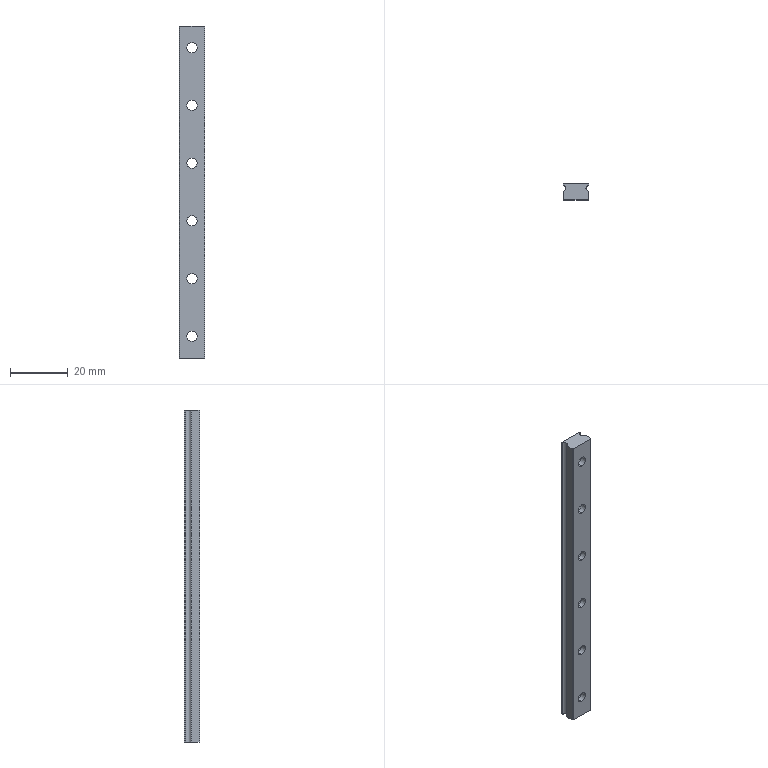Part | SolidWorks | features RefAxis 6, RevCut 6, 3DProfileFeature 2, Extrusion 1 | 1 solid | 43 faces | box 9 x 5.5 x 115 mm | volume 4582 mm3 | cylinder 27 | plane 16 | commonest cylinder face diameters 3.5 x12 6 x12 2.08 x3
STEP:
#1=CARTESIAN_POINT('',(0.,0.,25.75));
#2=VERTEX_POINT('',#1);
#3=CARTESIAN_POINT('',(0.,0.,29.25));
#4=VERTEX_POINT('',#3);
#5=CARTESIAN_POINT('',(0.,0.,27.5));
#6=DIRECTION('',(0.,1.,0.));
#7=DIRECTION('',(0.,0.,1.));
#8=AXIS2_PLACEMENT_3D('',#5,#6,#7);
#9=CIRCLE('',#8,1.75);
#10=EDGE_CURVE('',#2,#4,#9,.T.);
#11=ORIENTED_EDGE('',*,*,#10,.F.);
#12=CARTESIAN_POINT('',(0.,2.,25.75));
#13=VERTEX_POINT('',#12);
#14=CARTESIAN_POINT('',(0.,0.,25.75));
#15=DIRECTION('',(0.,1.,0.));
#16=VECTOR('',#15,1000.);
#17=LINE('',#14,#16);
#18=EDGE_CURVE('',#2,#13,#17,.T.);
#19=ORIENTED_EDGE('',*,*,#18,.T.);
#20=CARTESIAN_POINT('',(0.,2.,29.25));
#21=VERTEX_POINT('',#20);
#22=CARTESIAN_POINT('',(0.,2.,27.5));
#23=DIRECTION('',(0.,1.,0.));
#24=DIRECTION('',(0.,0.,1.));
#25=AXIS2_PLACEMENT_3D('',#22,#23,#24);
#26=CIRCLE('',#25,1.75);
#27=EDGE_CURVE('',#13,#21,#26,.T.);
#28=ORIENTED_EDGE('',*,*,#27,.T.);
#29=CARTESIAN_POINT('',(0.,0.,29.25));
#30=DIRECTION('',(0.,1.,0.));
#31=VECTOR('',#30,1000.);
#32=LINE('',#29,#31);
#33=EDGE_CURVE('',#4,#21,#32,.T.);
#34=ORIENTED_EDGE('',*,*,#33,.F.);
#35=EDGE_LOOP('',(#11,#19,#28,#34));
#36=FACE_OUTER_BOUND('',#35,.T.);
#37=CARTESIAN_POINT('',(0.,0.,27.5));
#38=DIRECTION('',(0.,1.,0.));
#39=DIRECTION('',(0.,0.,1.));
#40=AXIS2_PLACEMENT_3D('',#37,#38,#39);
#41=CYLINDRICAL_SURFACE('',#40,1.75);
#42=ADVANCED_FACE('',(#36),#41,.F.);
#43=CARTESIAN_POINT('',(0.,2.,24.5));
#44=VERTEX_POINT('',#43);
#45=CARTESIAN_POINT('',(0.,2.,30.5));
#46=VERTEX_POINT('',#45);
#47=CARTESIAN_POINT('',(0.,2.,27.5));
#48=DIRECTION('',(0.,1.,0.));
#49=DIRECTION('',(0.,0.,1.));
#50=AXIS2_PLACEMENT_3D('',#47,#48,#49);
#51=CIRCLE('',#50,3.);
#52=EDGE_CURVE('',#44,#46,#51,.T.);
#53=ORIENTED_EDGE('',*,*,#52,.F.);
#54=CARTESIAN_POINT('',(0.,5.5,24.5));
#55=VERTEX_POINT('',#54);
#56=CARTESIAN_POINT('',(0.,0.,24.5));
#57=DIRECTION('',(0.,1.,0.));
#58=VECTOR('',#57,1000.);
#59=LINE('',#56,#58);
#60=EDGE_CURVE('',#44,#55,#59,.T.);
#61=ORIENTED_EDGE('',*,*,#60,.T.);
#62=CARTESIAN_POINT('',(0.,5.5,30.5));
#63=VERTEX_POINT('',#62);
#64=CARTESIAN_POINT('',(0.,5.5,27.5));
#65=DIRECTION('',(0.,1.,0.));
#66=DIRECTION('',(0.,0.,1.));
#67=AXIS2_PLACEMENT_3D('',#64,#65,#66);
#68=CIRCLE('',#67,3.);
#69=EDGE_CURVE('',#55,#63,#68,.T.);
#70=ORIENTED_EDGE('',*,*,#69,.T.);
#71=CARTESIAN_POINT('',(0.,0.,30.5));
#72=DIRECTION('',(0.,1.,0.));
#73=VECTOR('',#72,1000.);
#74=LINE('',#71,#73);
#75=EDGE_CURVE('',#46,#63,#74,.T.);
#76=ORIENTED_EDGE('',*,*,#75,.F.);
#77=EDGE_LOOP('',(#53,#61,#70,#76));
#78=FACE_OUTER_BOUND('',#77,.T.);
#79=CARTESIAN_POINT('',(0.,0.,27.5));
#80=DIRECTION('',(0.,1.,0.));
#81=DIRECTION('',(0.,0.,1.));
#82=AXIS2_PLACEMENT_3D('',#79,#80,#81);
#83=CYLINDRICAL_SURFACE('',#82,3.);
#84=ADVANCED_FACE('',(#78),#83,.F.);
#85=CARTESIAN_POINT('',(0.,0.,45.75));
#86=VERTEX_POINT('',#85);
#87=CARTESIAN_POINT('',(0.,0.,49.25));
#88=VERTEX_POINT('',#87);
#89=CARTESIAN_POINT('',(0.,0.,47.5));
#90=DIRECTION('',(0.,1.,0.));
#91=DIRECTION('',(0.,0.,1.));
#92=AXIS2_PLACEMENT_3D('',#89,#90,#91);
#93=CIRCLE('',#92,1.75);
#94=EDGE_CURVE('',#86,#88,#93,.T.);
#95=ORIENTED_EDGE('',*,*,#94,.F.);
#96=CARTESIAN_POINT('',(0.,2.,45.75));
#97=VERTEX_POINT('',#96);
#98=CARTESIAN_POINT('',(0.,0.,45.75));
#99=DIRECTION('',(0.,1.,0.));
#100=VECTOR('',#99,1000.);
#101=LINE('',#98,#100);
#102=EDGE_CURVE('',#86,#97,#101,.T.);
#103=ORIENTED_EDGE('',*,*,#102,.T.);
#104=CARTESIAN_POINT('',(0.,2.,49.25));
#105=VERTEX_POINT('',#104);
#106=CARTESIAN_POINT('',(0.,2.,47.5));
#107=DIRECTION('',(0.,1.,0.));
#108=DIRECTION('',(0.,0.,1.));
#109=AXIS2_PLACEMENT_3D('',#106,#107,#108);
#110=CIRCLE('',#109,1.75);
#111=EDGE_CURVE('',#97,#105,#110,.T.);
#112=ORIENTED_EDGE('',*,*,#111,.T.);
#113=CARTESIAN_POINT('',(0.,0.,49.25));
#114=DIRECTION('',(0.,1.,0.));
#115=VECTOR('',#114,1000.);
#116=LINE('',#113,#115);
#117=EDGE_CURVE('',#88,#105,#116,.T.);
#118=ORIENTED_EDGE('',*,*,#117,.F.);
#119=EDGE_LOOP('',(#95,#103,#112,#118));
#120=FACE_OUTER_BOUND('',#119,.T.);
#121=CARTESIAN_POINT('',(0.,0.,47.5));
#122=DIRECTION('',(0.,1.,0.));
#123=DIRECTION('',(0.,0.,1.));
#124=AXIS2_PLACEMENT_3D('',#121,#122,#123);
#125=CYLINDRICAL_SURFACE('',#124,1.75);
#126=ADVANCED_FACE('',(#120),#125,.F.);
#127=CARTESIAN_POINT('',(0.,2.,44.5));
#128=VERTEX_POINT('',#127);
#129=CARTESIAN_POINT('',(0.,2.,50.5));
#130=VERTEX_POINT('',#129);
#131=CARTESIAN_POINT('',(0.,2.,47.5));
#132=DIRECTION('',(0.,1.,0.));
#133=DIRECTION('',(0.,0.,1.));
#134=AXIS2_PLACEMENT_3D('',#131,#132,#133);
#135=CIRCLE('',#134,3.);
#136=EDGE_CURVE('',#128,#130,#135,.T.);
#137=ORIENTED_EDGE('',*,*,#136,.F.);
#138=CARTESIAN_POINT('',(0.,5.5,44.5));
#139=VERTEX_POINT('',#138);
#140=CARTESIAN_POINT('',(0.,0.,44.5));
#141=DIRECTION('',(0.,1.,0.));
#142=VECTOR('',#141,1000.);
#143=LINE('',#140,#142);
#144=EDGE_CURVE('',#128,#139,#143,.T.);
#145=ORIENTED_EDGE('',*,*,#144,.T.);
#146=CARTESIAN_POINT('',(0.,5.5,50.5));
#147=VERTEX_POINT('',#146);
#148=CARTESIAN_POINT('',(0.,5.5,47.5));
#149=DIRECTION('',(0.,1.,0.));
#150=DIRECTION('',(0.,0.,1.));
#151=AXIS2_PLACEMENT_3D('',#148,#149,#150);
#152=CIRCLE('',#151,3.);
#153=EDGE_CURVE('',#139,#147,#152,.T.);
#154=ORIENTED_EDGE('',*,*,#153,.T.);
#155=CARTESIAN_POINT('',(0.,0.,50.5));
#156=DIRECTION('',(0.,1.,0.));
#157=VECTOR('',#156,1000.);
#158=LINE('',#155,#157);
#159=EDGE_CURVE('',#130,#147,#158,.T.);
#160=ORIENTED_EDGE('',*,*,#159,.F.);
#161=EDGE_LOOP('',(#137,#145,#154,#160));
#162=FACE_OUTER_BOUND('',#161,.T.);
#163=CARTESIAN_POINT('',(0.,0.,47.5));
#164=DIRECTION('',(0.,1.,0.));
#165=DIRECTION('',(0.,0.,1.));
#166=AXIS2_PLACEMENT_3D('',#163,#164,#165);
#167=CYLINDRICAL_SURFACE('',#166,3.);
#168=ADVANCED_FACE('',(#162),#167,.F.);
#169=CARTESIAN_POINT('',(0.,0.,65.75));
#170=VERTEX_POINT('',#169);
#171=CARTESIAN_POINT('',(0.,0.,69.25));
#172=VERTEX_POINT('',#171);
#173=CARTESIAN_POINT('',(0.,0.,67.5));
#174=DIRECTION('',(0.,1.,0.));
#175=DIRECTION('',(0.,0.,1.));
#176=AXIS2_PLACEMENT_3D('',#173,#174,#175);
#177=CIRCLE('',#176,1.75);
#178=EDGE_CURVE('',#170,#172,#177,.T.);
#179=ORIENTED_EDGE('',*,*,#178,.F.);
#180=CARTESIAN_POINT('',(0.,2.,65.75));
#181=VERTEX_POINT('',#180);
#182=CARTESIAN_POINT('',(0.,0.,65.75));
#183=DIRECTION('',(0.,1.,0.));
#184=VECTOR('',#183,1000.);
#185=LINE('',#182,#184);
#186=EDGE_CURVE('',#170,#181,#185,.T.);
#187=ORIENTED_EDGE('',*,*,#186,.T.);
#188=CARTESIAN_POINT('',(0.,2.,69.25));
#189=VERTEX_POINT('',#188);
#190=CARTESIAN_POINT('',(0.,2.,67.5));
#191=DIRECTION('',(0.,1.,0.));
#192=DIRECTION('',(0.,0.,1.));
#193=AXIS2_PLACEMENT_3D('',#190,#191,#192);
#194=CIRCLE('',#193,1.75);
#195=EDGE_CURVE('',#181,#189,#194,.T.);
#196=ORIENTED_EDGE('',*,*,#195,.T.);
#197=CARTESIAN_POINT('',(0.,0.,69.25));
#198=DIRECTION('',(0.,1.,0.));
#199=VECTOR('',#198,1000.);
#200=LINE('',#197,#199);
#201=EDGE_CURVE('',#172,#189,#200,.T.);
#202=ORIENTED_EDGE('',*,*,#201,.F.);
#203=EDGE_LOOP('',(#179,#187,#196,#202));
#204=FACE_OUTER_BOUND('',#203,.T.);
#205=CARTESIAN_POINT('',(0.,0.,67.5));
#206=DIRECTION('',(0.,1.,0.));
#207=DIRECTION('',(0.,0.,1.));
#208=AXIS2_PLACEMENT_3D('',#205,#206,#207);
#209=CYLINDRICAL_SURFACE('',#208,1.75);
#210=ADVANCED_FACE('',(#204),#209,.F.);
#211=CARTESIAN_POINT('',(0.,2.,64.5));
#212=VERTEX_POINT('',#211);
#213=CARTESIAN_POINT('',(0.,2.,70.5));
#214=VERTEX_POINT('',#213);
#215=CARTESIAN_POINT('',(0.,2.,67.5));
#216=DIRECTION('',(0.,1.,0.));
#217=DIRECTION('',(0.,0.,1.));
#218=AXIS2_PLACEMENT_3D('',#215,#216,#217);
#219=CIRCLE('',#218,3.);
#220=EDGE_CURVE('',#212,#214,#219,.T.);
#221=ORIENTED_EDGE('',*,*,#220,.F.);
#222=CARTESIAN_POINT('',(0.,5.5,64.5));
#223=VERTEX_POINT('',#222);
#224=CARTESIAN_POINT('',(0.,0.,64.5));
#225=DIRECTION('',(0.,1.,0.));
#226=VECTOR('',#225,1000.);
#227=LINE('',#224,#226);
#228=EDGE_CURVE('',#212,#223,#227,.T.);
#229=ORIENTED_EDGE('',*,*,#228,.T.);
#230=CARTESIAN_POINT('',(0.,5.5,70.5));
#231=VERTEX_POINT('',#230);
#232=CARTESIAN_POINT('',(0.,5.5,67.5));
#233=DIRECTION('',(0.,1.,0.));
#234=DIRECTION('',(0.,0.,1.));
#235=AXIS2_PLACEMENT_3D('',#232,#233,#234);
#236=CIRCLE('',#235,3.);
#237=EDGE_CURVE('',#223,#231,#236,.T.);
#238=ORIENTED_EDGE('',*,*,#237,.T.);
#239=CARTESIAN_POINT('',(0.,0.,70.5));
#240=DIRECTION('',(0.,1.,0.));
#241=VECTOR('',#240,1000.);
#242=LINE('',#239,#241);
#243=EDGE_CURVE('',#214,#231,#242,.T.);
#244=ORIENTED_EDGE('',*,*,#243,.F.);
#245=EDGE_LOOP('',(#221,#229,#238,#244));
#246=FACE_OUTER_BOUND('',#245,.T.);
#247=CARTESIAN_POINT('',(0.,0.,67.5));
#248=DIRECTION('',(0.,1.,0.));
#249=DIRECTION('',(0.,0.,1.));
#250=AXIS2_PLACEMENT_3D('',#247,#248,#249);
#251=CYLINDRICAL_SURFACE('',#250,3.);
#252=ADVANCED_FACE('',(#246),#251,.F.);
#253=CARTESIAN_POINT('',(0.,0.,85.75));
#254=VERTEX_POINT('',#253);
#255=CARTESIAN_POINT('',(0.,0.,89.25));
#256=VERTEX_POINT('',#255);
#257=CARTESIAN_POINT('',(0.,0.,87.5));
#258=DIRECTION('',(0.,1.,0.));
#259=DIRECTION('',(0.,0.,1.));
#260=AXIS2_PLACEMENT_3D('',#257,#258,#259);
#261=CIRCLE('',#260,1.75);
#262=EDGE_CURVE('',#254,#256,#261,.T.);
#263=ORIENTED_EDGE('',*,*,#262,.F.);
#264=CARTESIAN_POINT('',(0.,2.,85.75));
#265=VERTEX_POINT('',#264);
#266=CARTESIAN_POINT('',(0.,0.,85.75));
#267=DIRECTION('',(0.,1.,0.));
#268=VECTOR('',#267,1000.);
#269=LINE('',#266,#268);
#270=EDGE_CURVE('',#254,#265,#269,.T.);
#271=ORIENTED_EDGE('',*,*,#270,.T.);
#272=CARTESIAN_POINT('',(0.,2.,89.25));
#273=VERTEX_POINT('',#272);
#274=CARTESIAN_POINT('',(0.,2.,87.5));
#275=DIRECTION('',(0.,1.,0.));
#276=DIRECTION('',(0.,0.,1.));
#277=AXIS2_PLACEMENT_3D('',#274,#275,#276);
#278=CIRCLE('',#277,1.75);
#279=EDGE_CURVE('',#265,#273,#278,.T.);
#280=ORIENTED_EDGE('',*,*,#279,.T.);
#281=CARTESIAN_POINT('',(0.,0.,89.25));
#282=DIRECTION('',(0.,1.,0.));
#283=VECTOR('',#282,1000.);
#284=LINE('',#281,#283);
#285=EDGE_CURVE('',#256,#273,#284,.T.);
#286=ORIENTED_EDGE('',*,*,#285,.F.);
#287=EDGE_LOOP('',(#263,#271,#280,#286));
#288=FACE_OUTER_BOUND('',#287,.T.);
#289=CARTESIAN_POINT('',(0.,0.,87.5));
#290=DIRECTION('',(0.,1.,0.));
#291=DIRECTION('',(0.,0.,1.));
#292=AXIS2_PLACEMENT_3D('',#289,#290,#291);
#293=CYLINDRICAL_SURFACE('',#292,1.75);
#294=ADVANCED_FACE('',(#288),#293,.F.);
#295=CARTESIAN_POINT('',(0.,2.,84.5));
#296=VERTEX_POINT('',#295);
#297=CARTESIAN_POINT('',(0.,2.,90.5));
#298=VERTEX_POINT('',#297);
#299=CARTESIAN_POINT('',(0.,2.,87.5));
#300=DIRECTION('',(0.,1.,0.));
#301=DIRECTION('',(0.,0.,1.));
#302=AXIS2_PLACEMENT_3D('',#299,#300,#301);
#303=CIRCLE('',#302,3.);
#304=EDGE_CURVE('',#296,#298,#303,.T.);
#305=ORIENTED_EDGE('',*,*,#304,.F.);
#306=CARTESIAN_POINT('',(0.,5.5,84.5));
#307=VERTEX_POINT('',#306);
#308=CARTESIAN_POINT('',(0.,0.,84.5));
#309=DIRECTION('',(0.,1.,0.));
#310=VECTOR('',#309,1000.);
#311=LINE('',#308,#310);
#312=EDGE_CURVE('',#296,#307,#311,.T.);
#313=ORIENTED_EDGE('',*,*,#312,.T.);
#314=CARTESIAN_POINT('',(0.,5.5,90.5));
#315=VERTEX_POINT('',#314);
#316=CARTESIAN_POINT('',(0.,5.5,87.5));
#317=DIRECTION('',(0.,1.,0.));
#318=DIRECTION('',(0.,0.,1.));
#319=AXIS2_PLACEMENT_3D('',#316,#317,#318);
#320=CIRCLE('',#319,3.);
#321=EDGE_CURVE('',#307,#315,#320,.T.);
#322=ORIENTED_EDGE('',*,*,#321,.T.);
#323=CARTESIAN_POINT('',(0.,0.,90.5));
#324=DIRECTION('',(0.,1.,0.));
#325=VECTOR('',#324,1000.);
#326=LINE('',#323,#325);
#327=EDGE_CURVE('',#298,#315,#326,.T.);
#328=ORIENTED_EDGE('',*,*,#327,.F.);
#329=EDGE_LOOP('',(#305,#313,#322,#328));
#330=FACE_OUTER_BOUND('',#329,.T.);
#331=CARTESIAN_POINT('',(0.,0.,87.5));
#332=DIRECTION('',(0.,1.,0.));
#333=DIRECTION('',(0.,0.,1.));
#334=AXIS2_PLACEMENT_3D('',#331,#332,#333);
#335=CYLINDRICAL_SURFACE('',#334,3.);
#336=ADVANCED_FACE('',(#330),#335,.F.);
#337=CARTESIAN_POINT('',(0.,0.,105.75));
#338=VERTEX_POINT('',#337);
#339=CARTESIAN_POINT('',(0.,0.,109.25));
#340=VERTEX_POINT('',#339);
#341=CARTESIAN_POINT('',(0.,0.,107.5));
#342=DIRECTION('',(0.,1.,0.));
#343=DIRECTION('',(0.,0.,1.));
#344=AXIS2_PLACEMENT_3D('',#341,#342,#343);
#345=CIRCLE('',#344,1.75);
#346=EDGE_CURVE('',#338,#340,#345,.T.);
#347=ORIENTED_EDGE('',*,*,#346,.F.);
#348=CARTESIAN_POINT('',(0.,2.,105.75));
#349=VERTEX_POINT('',#348);
#350=CARTESIAN_POINT('',(0.,0.,105.75));
#351=DIRECTION('',(0.,1.,0.));
#352=VECTOR('',#351,1000.);
#353=LINE('',#350,#352);
#354=EDGE_CURVE('',#338,#349,#353,.T.);
#355=ORIENTED_EDGE('',*,*,#354,.T.);
#356=CARTESIAN_POINT('',(0.,2.,109.25));
#357=VERTEX_POINT('',#356);
#358=CARTESIAN_POINT('',(0.,2.,107.5));
#359=DIRECTION('',(0.,1.,0.));
#360=DIRECTION('',(0.,0.,1.));
#361=AXIS2_PLACEMENT_3D('',#358,#359,#360);
#362=CIRCLE('',#361,1.75);
#363=EDGE_CURVE('',#349,#357,#362,.T.);
#364=ORIENTED_EDGE('',*,*,#363,.T.);
#365=CARTESIAN_POINT('',(0.,0.,109.25));
#366=DIRECTION('',(0.,1.,0.));
#367=VECTOR('',#366,1000.);
#368=LINE('',#365,#367);
#369=EDGE_CURVE('',#340,#357,#368,.T.);
#370=ORIENTED_EDGE('',*,*,#369,.F.);
#371=EDGE_LOOP('',(#347,#355,#364,#370));
#372=FACE_OUTER_BOUND('',#371,.T.);
#373=CARTESIAN_POINT('',(0.,0.,107.5));
#374=DIRECTION('',(0.,1.,0.));
#375=DIRECTION('',(0.,0.,1.));
#376=AXIS2_PLACEMENT_3D('',#373,#374,#375);
#377=CYLINDRICAL_SURFACE('',#376,1.75);
#378=ADVANCED_FACE('',(#372),#377,.F.);
#379=CARTESIAN_POINT('',(0.,2.,104.5));
#380=VERTEX_POINT('',#379);
#381=CARTESIAN_POINT('',(0.,2.,110.5));
#382=VERTEX_POINT('',#381);
#383=CARTESIAN_POINT('',(0.,2.,107.5));
#384=DIRECTION('',(0.,1.,0.));
#385=DIRECTION('',(0.,0.,1.));
#386=AXIS2_PLACEMENT_3D('',#383,#384,#385);
#387=CIRCLE('',#386,3.);
#388=EDGE_CURVE('',#380,#382,#387,.T.);
#389=ORIENTED_EDGE('',*,*,#388,.F.);
#390=CARTESIAN_POINT('',(0.,5.5,104.5));
#391=VERTEX_POINT('',#390);
#392=CARTESIAN_POINT('',(0.,0.,104.5));
#393=DIRECTION('',(0.,1.,0.));
#394=VECTOR('',#393,1000.);
#395=LINE('',#392,#394);
#396=EDGE_CURVE('',#380,#391,#395,.T.);
#397=ORIENTED_EDGE('',*,*,#396,.T.);
#398=CARTESIAN_POINT('',(0.,5.5,110.5));
#399=VERTEX_POINT('',#398);
#400=CARTESIAN_POINT('',(0.,5.5,107.5));
#401=DIRECTION('',(0.,1.,0.));
#402=DIRECTION('',(0.,0.,1.));
#403=AXIS2_PLACEMENT_3D('',#400,#401,#402);
#404=CIRCLE('',#403,3.);
#405=EDGE_CURVE('',#391,#399,#404,.T.);
#406=ORIENTED_EDGE('',*,*,#405,.T.);
#407=CARTESIAN_POINT('',(0.,0.,110.5));
#408=DIRECTION('',(0.,1.,0.));
#409=VECTOR('',#408,1000.);
#410=LINE('',#407,#409);
#411=EDGE_CURVE('',#382,#399,#410,.T.);
#412=ORIENTED_EDGE('',*,*,#411,.F.);
#413=EDGE_LOOP('',(#389,#397,#406,#412));
#414=FACE_OUTER_BOUND('',#413,.T.);
#415=CARTESIAN_POINT('',(0.,0.,107.5));
#416=DIRECTION('',(0.,1.,0.));
#417=DIRECTION('',(0.,0.,1.));
#418=AXIS2_PLACEMENT_3D('',#415,#416,#417);
#419=CYLINDRICAL_SURFACE('',#418,3.);
#420=ADVANCED_FACE('',(#414),#419,.F.);
#421=CARTESIAN_POINT('',(0.,0.,5.75));
#422=VERTEX_POINT('',#421);
#423=CARTESIAN_POINT('',(0.,0.,9.25));
#424=VERTEX_POINT('',#423);
#425=CARTESIAN_POINT('',(0.,0.,7.5));
#426=DIRECTION('',(0.,1.,0.));
#427=DIRECTION('',(0.,0.,1.));
#428=AXIS2_PLACEMENT_3D('',#425,#426,#427);
#429=CIRCLE('',#428,1.75);
#430=EDGE_CURVE('',#422,#424,#429,.T.);
#431=ORIENTED_EDGE('',*,*,#430,.F.);
#432=CARTESIAN_POINT('',(0.,2.,5.75));
#433=VERTEX_POINT('',#432);
#434=CARTESIAN_POINT('',(0.,0.,5.75));
#435=DIRECTION('',(0.,1.,0.));
#436=VECTOR('',#435,1000.);
#437=LINE('',#434,#436);
#438=EDGE_CURVE('',#422,#433,#437,.T.);
#439=ORIENTED_EDGE('',*,*,#438,.T.);
#440=CARTESIAN_POINT('',(0.,2.,9.25));
#441=VERTEX_POINT('',#440);
#442=CARTESIAN_POINT('',(0.,2.,7.5));
#443=DIRECTION('',(0.,1.,0.));
#444=DIRECTION('',(0.,0.,1.));
#445=AXIS2_PLACEMENT_3D('',#442,#443,#444);
#446=CIRCLE('',#445,1.75);
#447=EDGE_CURVE('',#433,#441,#446,.T.);
#448=ORIENTED_EDGE('',*,*,#447,.T.);
#449=CARTESIAN_POINT('',(0.,0.,9.25));
#450=DIRECTION('',(0.,1.,0.));
#451=VECTOR('',#450,1000.);
#452=LINE('',#449,#451);
#453=EDGE_CURVE('',#424,#441,#452,.T.);
#454=ORIENTED_EDGE('',*,*,#453,.F.);
#455=EDGE_LOOP('',(#431,#439,#448,#454));
#456=FACE_OUTER_BOUND('',#455,.T.);
#457=CARTESIAN_POINT('',(0.,0.,7.5));
#458=DIRECTION('',(0.,1.,0.));
#459=DIRECTION('',(0.,0.,1.));
#460=AXIS2_PLACEMENT_3D('',#457,#458,#459);
#461=CYLINDRICAL_SURFACE('',#460,1.75);
#462=ADVANCED_FACE('',(#456),#461,.F.);
#463=CARTESIAN_POINT('',(0.,2.,4.5));
#464=VERTEX_POINT('',#463);
#465=CARTESIAN_POINT('',(0.,2.,10.5));
#466=VERTEX_POINT('',#465);
#467=CARTESIAN_POINT('',(0.,2.,7.5));
#468=DIRECTION('',(0.,1.,0.));
#469=DIRECTION('',(0.,0.,1.));
#470=AXIS2_PLACEMENT_3D('',#467,#468,#469);
#471=CIRCLE('',#470,3.);
#472=EDGE_CURVE('',#464,#466,#471,.T.);
#473=ORIENTED_EDGE('',*,*,#472,.F.);
#474=CARTESIAN_POINT('',(0.,5.5,4.5));
#475=VERTEX_POINT('',#474);
#476=CARTESIAN_POINT('',(0.,0.,4.5));
#477=DIRECTION('',(0.,1.,0.));
#478=VECTOR('',#477,1000.);
#479=LINE('',#476,#478);
#480=EDGE_CURVE('',#464,#475,#479,.T.);
#481=ORIENTED_EDGE('',*,*,#480,.T.);
#482=CARTESIAN_POINT('',(0.,5.5,10.5));
#483=VERTEX_POINT('',#482);
#484=CARTESIAN_POINT('',(0.,5.5,7.5));
#485=DIRECTION('',(0.,1.,0.));
#486=DIRECTION('',(0.,0.,1.));
#487=AXIS2_PLACEMENT_3D('',#484,#485,#486);
#488=CIRCLE('',#487,3.);
#489=EDGE_CURVE('',#475,#483,#488,.T.);
#490=ORIENTED_EDGE('',*,*,#489,.T.);
#491=CARTESIAN_POINT('',(0.,0.,10.5));
#492=DIRECTION('',(0.,1.,0.));
#493=VECTOR('',#492,1000.);
#494=LINE('',#491,#493);
#495=EDGE_CURVE('',#466,#483,#494,.T.);
#496=ORIENTED_EDGE('',*,*,#495,.F.);
#497=EDGE_LOOP('',(#473,#481,#490,#496));
#498=FACE_OUTER_BOUND('',#497,.T.);
#499=CARTESIAN_POINT('',(0.,0.,7.5));
#500=DIRECTION('',(0.,1.,0.));
#501=DIRECTION('',(0.,0.,1.));
#502=AXIS2_PLACEMENT_3D('',#499,#500,#501);
#503=CYLINDRICAL_SURFACE('',#502,3.);
#504=ADVANCED_FACE('',(#498),#503,.F.);
#505=CARTESIAN_POINT('',(3.46,4.,115.));
#506=VERTEX_POINT('',#505);
#507=CARTESIAN_POINT('',(4.5,5.04,115.));
#508=VERTEX_POINT('',#507);
#509=CARTESIAN_POINT('',(4.5,4.,115.));
#510=DIRECTION('',(0.,0.,-1.));
#511=DIRECTION('',(-1.,0.,0.));
#512=AXIS2_PLACEMENT_3D('',#509,#510,#511);
#513=CIRCLE('',#512,1.04);
#514=EDGE_CURVE('',#506,#508,#513,.T.);
#515=ORIENTED_EDGE('',*,*,#514,.F.);
#516=CARTESIAN_POINT('',(3.46,4.,0.));
#517=VERTEX_POINT('',#516);
#518=CARTESIAN_POINT('',(3.46,4.,115.));
#519=DIRECTION('',(0.,0.,-1.));
#520=VECTOR('',#519,1000.);
#521=LINE('',#518,#520);
#522=EDGE_CURVE('',#506,#517,#521,.T.);
#523=ORIENTED_EDGE('',*,*,#522,.T.);
#524=CARTESIAN_POINT('',(4.5,5.04,0.));
#525=VERTEX_POINT('',#524);
#526=CARTESIAN_POINT('',(4.5,4.,0.));
#527=DIRECTION('',(0.,0.,-1.));
#528=DIRECTION('',(-1.,0.,0.));
#529=AXIS2_PLACEMENT_3D('',#526,#527,#528);
#530=CIRCLE('',#529,1.04);
#531=EDGE_CURVE('',#517,#525,#530,.T.);
#532=ORIENTED_EDGE('',*,*,#531,.T.);
#533=CARTESIAN_POINT('',(4.5,5.04,115.));
#534=DIRECTION('',(0.,0.,-1.));
#535=VECTOR('',#534,1000.);
#536=LINE('',#533,#535);
#537=EDGE_CURVE('',#508,#525,#536,.T.);
#538=ORIENTED_EDGE('',*,*,#537,.F.);
#539=EDGE_LOOP('',(#515,#523,#532,#538));
#540=FACE_OUTER_BOUND('',#539,.T.);
#541=CARTESIAN_POINT('',(4.5,4.,115.));
#542=DIRECTION('',(0.,0.,-1.));
#543=DIRECTION('',(-1.,0.,0.));
#544=AXIS2_PLACEMENT_3D('',#541,#542,#543);
#545=CYLINDRICAL_SURFACE('',#544,1.04);
#546=ADVANCED_FACE('',(#540),#545,.F.);
#547=CARTESIAN_POINT('',(0.,5.5,47.5));
#548=DIRECTION('',(0.,1.,0.));
#549=DIRECTION('',(0.,0.,1.));
#550=AXIS2_PLACEMENT_3D('',#547,#548,#549);
#551=CIRCLE('',#550,3.);
#552=EDGE_CURVE('',#147,#139,#551,.T.);
#553=ORIENTED_EDGE('',*,*,#552,.F.);
#554=ORIENTED_EDGE('',*,*,#153,.F.);
#555=EDGE_LOOP('',(#553,#554));
#556=FACE_BOUND('',#555,.T.);
#557=CARTESIAN_POINT('',(0.,5.5,87.5));
#558=DIRECTION('',(0.,1.,0.));
#559=DIRECTION('',(0.,0.,1.));
#560=AXIS2_PLACEMENT_3D('',#557,#558,#559);
#561=CIRCLE('',#560,3.);
#562=EDGE_CURVE('',#315,#307,#561,.T.);
#563=ORIENTED_EDGE('',*,*,#562,.F.);
#564=ORIENTED_EDGE('',*,*,#321,.F.);
#565=EDGE_LOOP('',(#563,#564));
#566=FACE_BOUND('',#565,.T.);
#567=CARTESIAN_POINT('',(0.,5.5,7.5));
#568=DIRECTION('',(0.,1.,0.));
#569=DIRECTION('',(0.,0.,1.));
#570=AXIS2_PLACEMENT_3D('',#567,#568,#569);
#571=CIRCLE('',#570,3.);
#572=EDGE_CURVE('',#483,#475,#571,.T.);
#573=ORIENTED_EDGE('',*,*,#572,.F.);
#574=ORIENTED_EDGE('',*,*,#489,.F.);
#575=EDGE_LOOP('',(#573,#574));
#576=FACE_BOUND('',#575,.T.);
#577=CARTESIAN_POINT('',(4.5,5.5,0.));
#578=VERTEX_POINT('',#577);
#579=CARTESIAN_POINT('',(-4.5,5.5,0.));
#580=VERTEX_POINT('',#579);
#581=CARTESIAN_POINT('',(4.5,5.5,0.));
#582=DIRECTION('',(-1.,0.,0.));
#583=VECTOR('',#582,1000.);
#584=LINE('',#581,#583);
#585=EDGE_CURVE('',#578,#580,#584,.T.);
#586=ORIENTED_EDGE('',*,*,#585,.T.);
#587=CARTESIAN_POINT('',(-4.5,5.5,115.));
#588=VERTEX_POINT('',#587);
#589=CARTESIAN_POINT('',(-4.5,5.5,115.));
#590=DIRECTION('',(0.,0.,-1.));
#591=VECTOR('',#590,1000.);
#592=LINE('',#589,#591);
#593=EDGE_CURVE('',#588,#580,#592,.T.);
#594=ORIENTED_EDGE('',*,*,#593,.F.);
#595=CARTESIAN_POINT('',(4.5,5.5,115.));
#596=VERTEX_POINT('',#595);
#597=CARTESIAN_POINT('',(4.5,5.5,115.));
#598=DIRECTION('',(-1.,0.,0.));
#599=VECTOR('',#598,1000.);
#600=LINE('',#597,#599);
#601=EDGE_CURVE('',#596,#588,#600,.T.);
#602=ORIENTED_EDGE('',*,*,#601,.F.);
#603=CARTESIAN_POINT('',(4.5,5.5,115.));
#604=DIRECTION('',(0.,0.,-1.));
#605=VECTOR('',#604,1000.);
#606=LINE('',#603,#605);
#607=EDGE_CURVE('',#596,#578,#606,.T.);
#608=ORIENTED_EDGE('',*,*,#607,.T.);
#609=EDGE_LOOP('',(#586,#594,#602,#608));
#610=FACE_OUTER_BOUND('',#609,.T.);
#611=CARTESIAN_POINT('',(0.,5.5,107.5));
#612=DIRECTION('',(0.,1.,0.));
#613=DIRECTION('',(0.,0.,1.));
#614=AXIS2_PLACEMENT_3D('',#611,#612,#613);
#615=CIRCLE('',#614,3.);
#616=EDGE_CURVE('',#399,#391,#615,.T.);
#617=ORIENTED_EDGE('',*,*,#616,.F.);
#618=ORIENTED_EDGE('',*,*,#405,.F.);
#619=EDGE_LOOP('',(#617,#618));
#620=FACE_BOUND('',#619,.T.);
#621=CARTESIAN_POINT('',(0.,5.5,67.5));
#622=DIRECTION('',(0.,1.,0.));
#623=DIRECTION('',(0.,0.,1.));
#624=AXIS2_PLACEMENT_3D('',#621,#622,#623);
#625=CIRCLE('',#624,3.);
#626=EDGE_CURVE('',#231,#223,#625,.T.);
#627=ORIENTED_EDGE('',*,*,#626,.F.);
#628=ORIENTED_EDGE('',*,*,#237,.F.);
#629=EDGE_LOOP('',(#627,#628));
#630=FACE_BOUND('',#629,.T.);
#631=CARTESIAN_POINT('',(0.,5.5,27.5));
#632=DIRECTION('',(0.,1.,0.));
#633=DIRECTION('',(0.,0.,1.));
#634=AXIS2_PLACEMENT_3D('',#631,#632,#633);
#635=CIRCLE('',#634,3.);
#636=EDGE_CURVE('',#63,#55,#635,.T.);
#637=ORIENTED_EDGE('',*,*,#636,.F.);
#638=ORIENTED_EDGE('',*,*,#69,.F.);
#639=EDGE_LOOP('',(#637,#638));
#640=FACE_BOUND('',#639,.T.);
#641=CARTESIAN_POINT('',(4.5,5.5,115.));
#642=DIRECTION('',(0.,-1.,0.));
#643=DIRECTION('',(0.,0.,-1.));
#644=AXIS2_PLACEMENT_3D('',#641,#642,#643);
#645=PLANE('',#644);
#646=ADVANCED_FACE('',(#556,#566,#576,#610,#620,#630,#640),#645,.F.);
#647=CARTESIAN_POINT('',(0.,0.,47.5));
#648=DIRECTION('',(0.,1.,0.));
#649=DIRECTION('',(0.,0.,1.));
#650=AXIS2_PLACEMENT_3D('',#647,#648,#649);
#651=CIRCLE('',#650,1.75);
#652=EDGE_CURVE('',#88,#86,#651,.T.);
#653=ORIENTED_EDGE('',*,*,#652,.T.);
#654=ORIENTED_EDGE('',*,*,#94,.T.);
#655=EDGE_LOOP('',(#653,#654));
#656=FACE_BOUND('',#655,.T.);
#657=CARTESIAN_POINT('',(0.,0.,87.5));
#658=DIRECTION('',(0.,1.,0.));
#659=DIRECTION('',(0.,0.,1.));
#660=AXIS2_PLACEMENT_3D('',#657,#658,#659);
#661=CIRCLE('',#660,1.75);
#662=EDGE_CURVE('',#256,#254,#661,.T.);
#663=ORIENTED_EDGE('',*,*,#662,.T.);
#664=ORIENTED_EDGE('',*,*,#262,.T.);
#665=EDGE_LOOP('',(#663,#664));
#666=FACE_BOUND('',#665,.T.);
#667=CARTESIAN_POINT('',(0.,0.,7.5));
#668=DIRECTION('',(0.,1.,0.));
#669=DIRECTION('',(0.,0.,1.));
#670=AXIS2_PLACEMENT_3D('',#667,#668,#669);
#671=CIRCLE('',#670,1.75);
#672=EDGE_CURVE('',#424,#422,#671,.T.);
#673=ORIENTED_EDGE('',*,*,#672,.T.);
#674=ORIENTED_EDGE('',*,*,#430,.T.);
#675=EDGE_LOOP('',(#673,#674));
#676=FACE_BOUND('',#675,.T.);
#677=CARTESIAN_POINT('',(-4.203,0.,0.));
#678=VERTEX_POINT('',#677);
#679=CARTESIAN_POINT('',(4.203,0.,0.));
#680=VERTEX_POINT('',#679);
#681=CARTESIAN_POINT('',(-4.203,0.,0.));
#682=DIRECTION('',(1.,0.,0.));
#683=VECTOR('',#682,1000.);
#684=LINE('',#681,#683);
#685=EDGE_CURVE('',#678,#680,#684,.T.);
#686=ORIENTED_EDGE('',*,*,#685,.T.);
#687=CARTESIAN_POINT('',(4.203,0.,115.));
#688=VERTEX_POINT('',#687);
#689=CARTESIAN_POINT('',(4.203,0.,115.));
#690=DIRECTION('',(0.,0.,-1.));
#691=VECTOR('',#690,1000.);
#692=LINE('',#689,#691);
#693=EDGE_CURVE('',#688,#680,#692,.T.);
#694=ORIENTED_EDGE('',*,*,#693,.F.);
#695=CARTESIAN_POINT('',(-4.203,0.,115.));
#696=VERTEX_POINT('',#695);
#697=CARTESIAN_POINT('',(-4.203,0.,115.));
#698=DIRECTION('',(1.,0.,0.));
#699=VECTOR('',#698,1000.);
#700=LINE('',#697,#699);
#701=EDGE_CURVE('',#696,#688,#700,.T.);
#702=ORIENTED_EDGE('',*,*,#701,.F.);
#703=CARTESIAN_POINT('',(-4.203,0.,115.));
#704=DIRECTION('',(0.,0.,-1.));
#705=VECTOR('',#704,1000.);
#706=LINE('',#703,#705);
#707=EDGE_CURVE('',#696,#678,#706,.T.);
#708=ORIENTED_EDGE('',*,*,#707,.T.);
#709=EDGE_LOOP('',(#686,#694,#702,#708));
#710=FACE_OUTER_BOUND('',#709,.T.);
#711=CARTESIAN_POINT('',(0.,0.,107.5));
#712=DIRECTION('',(0.,1.,0.));
#713=DIRECTION('',(0.,0.,1.));
#714=AXIS2_PLACEMENT_3D('',#711,#712,#713);
#715=CIRCLE('',#714,1.75);
#716=EDGE_CURVE('',#340,#338,#715,.T.);
#717=ORIENTED_EDGE('',*,*,#716,.T.);
#718=ORIENTED_EDGE('',*,*,#346,.T.);
#719=EDGE_LOOP('',(#717,#718));
#720=FACE_BOUND('',#719,.T.);
#721=CARTESIAN_POINT('',(0.,0.,67.5));
#722=DIRECTION('',(0.,1.,0.));
#723=DIRECTION('',(0.,0.,1.));
#724=AXIS2_PLACEMENT_3D('',#721,#722,#723);
#725=CIRCLE('',#724,1.75);
#726=EDGE_CURVE('',#172,#170,#725,.T.);
#727=ORIENTED_EDGE('',*,*,#726,.T.);
#728=ORIENTED_EDGE('',*,*,#178,.T.);
#729=EDGE_LOOP('',(#727,#728));
#730=FACE_BOUND('',#729,.T.);
#731=CARTESIAN_POINT('',(0.,0.,27.5));
#732=DIRECTION('',(0.,1.,0.));
#733=DIRECTION('',(0.,0.,1.));
#734=AXIS2_PLACEMENT_3D('',#731,#732,#733);
#735=CIRCLE('',#734,1.75);
#736=EDGE_CURVE('',#4,#2,#735,.T.);
#737=ORIENTED_EDGE('',*,*,#736,.T.);
#738=ORIENTED_EDGE('',*,*,#10,.T.);
#739=EDGE_LOOP('',(#737,#738));
#740=FACE_BOUND('',#739,.T.);
#741=CARTESIAN_POINT('',(-4.203,0.,115.));
#742=DIRECTION('',(0.,1.,0.));
#743=DIRECTION('',(0.,0.,1.));
#744=AXIS2_PLACEMENT_3D('',#741,#742,#743);
#745=PLANE('',#744);
#746=ADVANCED_FACE('',(#656,#666,#676,#710,#720,#730,#740),#745,.F.);
#747=CARTESIAN_POINT('',(-4.5,5.04,0.));
#748=VERTEX_POINT('',#747);
#749=CARTESIAN_POINT('',(-4.5,5.5,0.));
#750=DIRECTION('',(0.,-1.,0.));
#751=VECTOR('',#750,1000.);
#752=LINE('',#749,#751);
#753=EDGE_CURVE('',#580,#748,#752,.T.);
#754=ORIENTED_EDGE('',*,*,#753,.T.);
#755=CARTESIAN_POINT('',(-4.5,5.04,115.));
#756=VERTEX_POINT('',#755);
#757=CARTESIAN_POINT('',(-4.5,5.04,115.));
#758=DIRECTION('',(0.,0.,-1.));
#759=VECTOR('',#758,1000.);
#760=LINE('',#757,#759);
#761=EDGE_CURVE('',#756,#748,#760,.T.);
#762=ORIENTED_EDGE('',*,*,#761,.F.);
#763=CARTESIAN_POINT('',(-4.5,5.5,115.));
#764=DIRECTION('',(0.,-1.,0.));
#765=VECTOR('',#764,1000.);
#766=LINE('',#763,#765);
#767=EDGE_CURVE('',#588,#756,#766,.T.);
#768=ORIENTED_EDGE('',*,*,#767,.F.);
#769=ORIENTED_EDGE('',*,*,#593,.T.);
#770=EDGE_LOOP('',(#754,#762,#768,#769));
#771=FACE_OUTER_BOUND('',#770,.T.);
#772=CARTESIAN_POINT('',(-4.5,5.5,115.));
#773=DIRECTION('',(1.,0.,0.));
#774=DIRECTION('',(0.,0.,-1.));
#775=AXIS2_PLACEMENT_3D('',#772,#773,#774);
#776=PLANE('',#775);
#777=ADVANCED_FACE('',(#771),#776,.F.);
#778=CARTESIAN_POINT('',(-4.5,2.96,0.));
#779=VERTEX_POINT('',#778);
#780=CARTESIAN_POINT('',(-4.5,4.,0.));
#781=DIRECTION('',(0.,0.,-1.));
#782=DIRECTION('',(-1.,0.,0.));
#783=AXIS2_PLACEMENT_3D('',#780,#781,#782);
#784=CIRCLE('',#783,1.04);
#785=EDGE_CURVE('',#748,#779,#784,.T.);
#786=ORIENTED_EDGE('',*,*,#785,.T.);
#787=CARTESIAN_POINT('',(-4.5,2.96,115.));
#788=VERTEX_POINT('',#787);
#789=CARTESIAN_POINT('',(-4.5,2.96,115.));
#790=DIRECTION('',(0.,0.,-1.));
#791=VECTOR('',#790,1000.);
#792=LINE('',#789,#791);
#793=EDGE_CURVE('',#788,#779,#792,.T.);
#794=ORIENTED_EDGE('',*,*,#793,.F.);
#795=CARTESIAN_POINT('',(-4.5,4.,115.));
#796=DIRECTION('',(0.,0.,-1.));
#797=DIRECTION('',(-1.,0.,0.));
#798=AXIS2_PLACEMENT_3D('',#795,#796,#797);
#799=CIRCLE('',#798,1.04);
#800=EDGE_CURVE('',#756,#788,#799,.T.);
#801=ORIENTED_EDGE('',*,*,#800,.F.);
#802=ORIENTED_EDGE('',*,*,#761,.T.);
#803=EDGE_LOOP('',(#786,#794,#801,#802));
#804=FACE_OUTER_BOUND('',#803,.T.);
#805=CARTESIAN_POINT('',(-4.5,4.,115.));
#806=DIRECTION('',(0.,0.,-1.));
#807=DIRECTION('',(-1.,0.,0.));
#808=AXIS2_PLACEMENT_3D('',#805,#806,#807);
#809=CYLINDRICAL_SURFACE('',#808,1.04);
#810=ADVANCED_FACE('',(#804),#809,.F.);
#811=CARTESIAN_POINT('',(-4.5,0.297,0.));
#812=VERTEX_POINT('',#811);
#813=CARTESIAN_POINT('',(-4.5,2.96,0.));
#814=DIRECTION('',(0.,-1.,0.));
#815=VECTOR('',#814,1000.);
#816=LINE('',#813,#815);
#817=EDGE_CURVE('',#779,#812,#816,.T.);
#818=ORIENTED_EDGE('',*,*,#817,.T.);
#819=CARTESIAN_POINT('',(-4.5,0.297,115.));
#820=VERTEX_POINT('',#819);
#821=CARTESIAN_POINT('',(-4.5,0.297,115.));
#822=DIRECTION('',(0.,0.,-1.));
#823=VECTOR('',#822,1000.);
#824=LINE('',#821,#823);
#825=EDGE_CURVE('',#820,#812,#824,.T.);
#826=ORIENTED_EDGE('',*,*,#825,.F.);
#827=CARTESIAN_POINT('',(-4.5,2.96,115.));
#828=DIRECTION('',(0.,-1.,0.));
#829=VECTOR('',#828,1000.);
#830=LINE('',#827,#829);
#831=EDGE_CURVE('',#788,#820,#830,.T.);
#832=ORIENTED_EDGE('',*,*,#831,.F.);
#833=ORIENTED_EDGE('',*,*,#793,.T.);
#834=EDGE_LOOP('',(#818,#826,#832,#833));
#835=FACE_OUTER_BOUND('',#834,.T.);
#836=CARTESIAN_POINT('',(-4.5,2.96,115.));
#837=DIRECTION('',(1.,0.,0.));
#838=DIRECTION('',(0.,0.,-1.));
#839=AXIS2_PLACEMENT_3D('',#836,#837,#838);
#840=PLANE('',#839);
#841=ADVANCED_FACE('',(#835),#840,.F.);
#842=CARTESIAN_POINT('',(-4.5,0.297,0.));
#843=DIRECTION('',(0.7071,-0.7071,0.));
#844=VECTOR('',#843,1000.);
#845=LINE('',#842,#844);
#846=EDGE_CURVE('',#812,#678,#845,.T.);
#847=ORIENTED_EDGE('',*,*,#846,.T.);
#848=ORIENTED_EDGE('',*,*,#707,.F.);
#849=CARTESIAN_POINT('',(-4.5,0.297,115.));
#850=DIRECTION('',(0.7071,-0.7071,0.));
#851=VECTOR('',#850,1000.);
#852=LINE('',#849,#851);
#853=EDGE_CURVE('',#820,#696,#852,.T.);
#854=ORIENTED_EDGE('',*,*,#853,.F.);
#855=ORIENTED_EDGE('',*,*,#825,.T.);
#856=EDGE_LOOP('',(#847,#848,#854,#855));
#857=FACE_OUTER_BOUND('',#856,.T.);
#858=CARTESIAN_POINT('',(-4.5,0.297,115.));
#859=DIRECTION('',(0.7071,0.7071,0.));
#860=DIRECTION('',(-0.7071,0.7071,0.));
#861=AXIS2_PLACEMENT_3D('',#858,#859,#860);
#862=PLANE('',#861);
#863=ADVANCED_FACE('',(#857),#862,.F.);
#864=CARTESIAN_POINT('',(4.5,0.297,0.));
#865=VERTEX_POINT('',#864);
#866=CARTESIAN_POINT('',(4.203,0.,0.));
#867=DIRECTION('',(0.7071,0.7071,0.));
#868=VECTOR('',#867,1000.);
#869=LINE('',#866,#868);
#870=EDGE_CURVE('',#680,#865,#869,.T.);
#871=ORIENTED_EDGE('',*,*,#870,.T.);
#872=CARTESIAN_POINT('',(4.5,0.297,115.));
#873=VERTEX_POINT('',#872);
#874=CARTESIAN_POINT('',(4.5,0.297,115.));
#875=DIRECTION('',(0.,0.,-1.));
#876=VECTOR('',#875,1000.);
#877=LINE('',#874,#876);
#878=EDGE_CURVE('',#873,#865,#877,.T.);
#879=ORIENTED_EDGE('',*,*,#878,.F.);
#880=CARTESIAN_POINT('',(4.203,0.,115.));
#881=DIRECTION('',(0.7071,0.7071,0.));
#882=VECTOR('',#881,1000.);
#883=LINE('',#880,#882);
#884=EDGE_CURVE('',#688,#873,#883,.T.);
#885=ORIENTED_EDGE('',*,*,#884,.F.);
#886=ORIENTED_EDGE('',*,*,#693,.T.);
#887=EDGE_LOOP('',(#871,#879,#885,#886));
#888=FACE_OUTER_BOUND('',#887,.T.);
#889=CARTESIAN_POINT('',(4.203,0.,115.));
#890=DIRECTION('',(-0.7071,0.7071,0.));
#891=DIRECTION('',(-0.7071,-0.7071,0.));
#892=AXIS2_PLACEMENT_3D('',#889,#890,#891);
#893=PLANE('',#892);
#894=ADVANCED_FACE('',(#888),#893,.F.);
#895=CARTESIAN_POINT('',(4.5,2.96,0.));
#896=VERTEX_POINT('',#895);
#897=CARTESIAN_POINT('',(4.5,0.297,0.));
#898=DIRECTION('',(0.,1.,0.));
#899=VECTOR('',#898,1000.);
#900=LINE('',#897,#899);
#901=EDGE_CURVE('',#865,#896,#900,.T.);
#902=ORIENTED_EDGE('',*,*,#901,.T.);
#903=CARTESIAN_POINT('',(4.5,2.96,115.));
#904=VERTEX_POINT('',#903);
#905=CARTESIAN_POINT('',(4.5,2.96,115.));
#906=DIRECTION('',(0.,0.,-1.));
#907=VECTOR('',#906,1000.);
#908=LINE('',#905,#907);
#909=EDGE_CURVE('',#904,#896,#908,.T.);
#910=ORIENTED_EDGE('',*,*,#909,.F.);
#911=CARTESIAN_POINT('',(4.5,0.297,115.));
#912=DIRECTION('',(0.,1.,0.));
#913=VECTOR('',#912,1000.);
#914=LINE('',#911,#913);
#915=EDGE_CURVE('',#873,#904,#914,.T.);
#916=ORIENTED_EDGE('',*,*,#915,.F.);
#917=ORIENTED_EDGE('',*,*,#878,.T.);
#918=EDGE_LOOP('',(#902,#910,#916,#917));
#919=FACE_OUTER_BOUND('',#918,.T.);
#920=CARTESIAN_POINT('',(4.5,0.297,115.));
#921=DIRECTION('',(-1.,0.,0.));
#922=DIRECTION('',(0.,0.,1.));
#923=AXIS2_PLACEMENT_3D('',#920,#921,#922);
#924=PLANE('',#923);
#925=ADVANCED_FACE('',(#919),#924,.F.);
#926=ORIENTED_EDGE('',*,*,#522,.F.);
#927=CARTESIAN_POINT('',(4.5,4.,115.));
#928=DIRECTION('',(0.,0.,-1.));
#929=DIRECTION('',(-1.,0.,0.));
#930=AXIS2_PLACEMENT_3D('',#927,#928,#929);
#931=CIRCLE('',#930,1.04);
#932=EDGE_CURVE('',#904,#506,#931,.T.);
#933=ORIENTED_EDGE('',*,*,#932,.F.);
#934=ORIENTED_EDGE('',*,*,#909,.T.);
#935=CARTESIAN_POINT('',(4.5,4.,0.));
#936=DIRECTION('',(0.,0.,-1.));
#937=DIRECTION('',(-1.,0.,0.));
#938=AXIS2_PLACEMENT_3D('',#935,#936,#937);
#939=CIRCLE('',#938,1.04);
#940=EDGE_CURVE('',#896,#517,#939,.T.);
#941=ORIENTED_EDGE('',*,*,#940,.T.);
#942=EDGE_LOOP('',(#926,#933,#934,#941));
#943=FACE_OUTER_BOUND('',#942,.T.);
#944=CARTESIAN_POINT('',(4.5,4.,115.));
#945=DIRECTION('',(0.,0.,-1.));
#946=DIRECTION('',(-1.,0.,0.));
#947=AXIS2_PLACEMENT_3D('',#944,#945,#946);
#948=CYLINDRICAL_SURFACE('',#947,1.04);
#949=ADVANCED_FACE('',(#943),#948,.F.);
#950=CARTESIAN_POINT('',(4.5,5.04,0.));
#951=DIRECTION('',(0.,1.,0.));
#952=VECTOR('',#951,1000.);
#953=LINE('',#950,#952);
#954=EDGE_CURVE('',#525,#578,#953,.T.);
#955=ORIENTED_EDGE('',*,*,#954,.T.);
#956=ORIENTED_EDGE('',*,*,#607,.F.);
#957=CARTESIAN_POINT('',(4.5,5.04,115.));
#958=DIRECTION('',(0.,1.,0.));
#959=VECTOR('',#958,1000.);
#960=LINE('',#957,#959);
#961=EDGE_CURVE('',#508,#596,#960,.T.);
#962=ORIENTED_EDGE('',*,*,#961,.F.);
#963=ORIENTED_EDGE('',*,*,#537,.T.);
#964=EDGE_LOOP('',(#955,#956,#962,#963));
#965=FACE_OUTER_BOUND('',#964,.T.);
#966=CARTESIAN_POINT('',(4.5,5.04,115.));
#967=DIRECTION('',(-1.,0.,0.));
#968=DIRECTION('',(0.,0.,1.));
#969=AXIS2_PLACEMENT_3D('',#966,#967,#968);
#970=PLANE('',#969);
#971=ADVANCED_FACE('',(#965),#970,.F.);
#972=ORIENTED_EDGE('',*,*,#601,.T.);
#973=ORIENTED_EDGE('',*,*,#767,.T.);
#974=ORIENTED_EDGE('',*,*,#800,.T.);
#975=ORIENTED_EDGE('',*,*,#831,.T.);
#976=ORIENTED_EDGE('',*,*,#853,.T.);
#977=ORIENTED_EDGE('',*,*,#701,.T.);
#978=ORIENTED_EDGE('',*,*,#884,.T.);
#979=ORIENTED_EDGE('',*,*,#915,.T.);
#980=ORIENTED_EDGE('',*,*,#932,.T.);
#981=ORIENTED_EDGE('',*,*,#514,.T.);
#982=ORIENTED_EDGE('',*,*,#961,.T.);
#983=EDGE_LOOP('',(#972,#973,#974,#975,#976,#977,#978,#979,#980,#981,#982));
#984=FACE_OUTER_BOUND('',#983,.T.);
#985=CARTESIAN_POINT('',(-4.5,4.,115.));
#986=DIRECTION('',(0.,0.,-1.));
#987=DIRECTION('',(-1.,0.,0.));
#988=AXIS2_PLACEMENT_3D('',#985,#986,#987);
#989=PLANE('',#988);
#990=ADVANCED_FACE('',(#984),#989,.F.);
#991=ORIENTED_EDGE('',*,*,#585,.F.);
#992=ORIENTED_EDGE('',*,*,#954,.F.);
#993=ORIENTED_EDGE('',*,*,#531,.F.);
#994=ORIENTED_EDGE('',*,*,#940,.F.);
#995=ORIENTED_EDGE('',*,*,#901,.F.);
#996=ORIENTED_EDGE('',*,*,#870,.F.);
#997=ORIENTED_EDGE('',*,*,#685,.F.);
#998=ORIENTED_EDGE('',*,*,#846,.F.);
#999=ORIENTED_EDGE('',*,*,#817,.F.);
#1000=ORIENTED_EDGE('',*,*,#785,.F.);
#1001=ORIENTED_EDGE('',*,*,#753,.F.);
#1002=EDGE_LOOP('',(#991,#992,#993,#994,#995,#996,#997,#998,#999,#1000,#1001));
#1003=FACE_OUTER_BOUND('',#1002,.T.);
#1004=CARTESIAN_POINT('',(-4.5,4.,0.));
#1005=DIRECTION('',(0.,0.,-1.));
#1006=DIRECTION('',(-1.,0.,0.));
#1007=AXIS2_PLACEMENT_3D('',#1004,#1005,#1006);
#1008=PLANE('',#1007);
#1009=ADVANCED_FACE('',(#1003),#1008,.T.);
#1010=ORIENTED_EDGE('',*,*,#480,.F.);
#1011=CARTESIAN_POINT('',(0.,2.,7.5));
#1012=DIRECTION('',(0.,1.,0.));
#1013=DIRECTION('',(0.,0.,1.));
#1014=AXIS2_PLACEMENT_3D('',#1011,#1012,#1013);
#1015=CIRCLE('',#1014,3.);
#1016=EDGE_CURVE('',#466,#464,#1015,.T.);
#1017=ORIENTED_EDGE('',*,*,#1016,.F.);
#1018=ORIENTED_EDGE('',*,*,#495,.T.);
#1019=ORIENTED_EDGE('',*,*,#572,.T.);
#1020=EDGE_LOOP('',(#1010,#1017,#1018,#1019));
#1021=FACE_OUTER_BOUND('',#1020,.T.);
#1022=CARTESIAN_POINT('',(0.,0.,7.5));
#1023=DIRECTION('',(0.,1.,0.));
#1024=DIRECTION('',(0.,0.,1.));
#1025=AXIS2_PLACEMENT_3D('',#1022,#1023,#1024);
#1026=CYLINDRICAL_SURFACE('',#1025,3.);
#1027=ADVANCED_FACE('',(#1021),#1026,.F.);
#1028=ORIENTED_EDGE('',*,*,#1016,.T.);
#1029=ORIENTED_EDGE('',*,*,#472,.T.);
#1030=EDGE_LOOP('',(#1028,#1029));
#1031=FACE_OUTER_BOUND('',#1030,.T.);
#1032=CARTESIAN_POINT('',(0.,2.,7.5));
#1033=DIRECTION('',(0.,1.,0.));
#1034=DIRECTION('',(0.,0.,1.));
#1035=AXIS2_PLACEMENT_3D('',#1032,#1033,#1034);
#1036=CIRCLE('',#1035,1.75);
#1037=EDGE_CURVE('',#441,#433,#1036,.T.);
#1038=ORIENTED_EDGE('',*,*,#1037,.F.);
#1039=ORIENTED_EDGE('',*,*,#447,.F.);
#1040=EDGE_LOOP('',(#1038,#1039));
#1041=FACE_BOUND('',#1040,.T.);
#1042=CARTESIAN_POINT('',(0.,2.,4.5));
#1043=DIRECTION('',(0.,1.,0.));
#1044=DIRECTION('',(0.,0.,1.));
#1045=AXIS2_PLACEMENT_3D('',#1042,#1043,#1044);
#1046=PLANE('',#1045);
#1047=ADVANCED_FACE('',(#1031,#1041),#1046,.T.);
#1048=ORIENTED_EDGE('',*,*,#438,.F.);
#1049=ORIENTED_EDGE('',*,*,#672,.F.);
#1050=ORIENTED_EDGE('',*,*,#453,.T.);
#1051=ORIENTED_EDGE('',*,*,#1037,.T.);
#1052=EDGE_LOOP('',(#1048,#1049,#1050,#1051));
#1053=FACE_OUTER_BOUND('',#1052,.T.);
#1054=CARTESIAN_POINT('',(0.,0.,7.5));
#1055=DIRECTION('',(0.,1.,0.));
#1056=DIRECTION('',(0.,0.,1.));
#1057=AXIS2_PLACEMENT_3D('',#1054,#1055,#1056);
#1058=CYLINDRICAL_SURFACE('',#1057,1.75);
#1059=ADVANCED_FACE('',(#1053),#1058,.F.);
#1060=ORIENTED_EDGE('',*,*,#396,.F.);
#1061=CARTESIAN_POINT('',(0.,2.,107.5));
#1062=DIRECTION('',(0.,1.,0.));
#1063=DIRECTION('',(0.,0.,1.));
#1064=AXIS2_PLACEMENT_3D('',#1061,#1062,#1063);
#1065=CIRCLE('',#1064,3.);
#1066=EDGE_CURVE('',#382,#380,#1065,.T.);
#1067=ORIENTED_EDGE('',*,*,#1066,.F.);
#1068=ORIENTED_EDGE('',*,*,#411,.T.);
#1069=ORIENTED_EDGE('',*,*,#616,.T.);
#1070=EDGE_LOOP('',(#1060,#1067,#1068,#1069));
#1071=FACE_OUTER_BOUND('',#1070,.T.);
#1072=CARTESIAN_POINT('',(0.,0.,107.5));
#1073=DIRECTION('',(0.,1.,0.));
#1074=DIRECTION('',(0.,0.,1.));
#1075=AXIS2_PLACEMENT_3D('',#1072,#1073,#1074);
#1076=CYLINDRICAL_SURFACE('',#1075,3.);
#1077=ADVANCED_FACE('',(#1071),#1076,.F.);
#1078=ORIENTED_EDGE('',*,*,#1066,.T.);
#1079=ORIENTED_EDGE('',*,*,#388,.T.);
#1080=EDGE_LOOP('',(#1078,#1079));
#1081=FACE_OUTER_BOUND('',#1080,.T.);
#1082=CARTESIAN_POINT('',(0.,2.,107.5));
#1083=DIRECTION('',(0.,1.,0.));
#1084=DIRECTION('',(0.,0.,1.));
#1085=AXIS2_PLACEMENT_3D('',#1082,#1083,#1084);
#1086=CIRCLE('',#1085,1.75);
#1087=EDGE_CURVE('',#357,#349,#1086,.T.);
#1088=ORIENTED_EDGE('',*,*,#1087,.F.);
#1089=ORIENTED_EDGE('',*,*,#363,.F.);
#1090=EDGE_LOOP('',(#1088,#1089));
#1091=FACE_BOUND('',#1090,.T.);
#1092=CARTESIAN_POINT('',(0.,2.,104.5));
#1093=DIRECTION('',(0.,1.,0.));
#1094=DIRECTION('',(0.,0.,1.));
#1095=AXIS2_PLACEMENT_3D('',#1092,#1093,#1094);
#1096=PLANE('',#1095);
#1097=ADVANCED_FACE('',(#1081,#1091),#1096,.T.);
#1098=ORIENTED_EDGE('',*,*,#354,.F.);
#1099=ORIENTED_EDGE('',*,*,#716,.F.);
#1100=ORIENTED_EDGE('',*,*,#369,.T.);
#1101=ORIENTED_EDGE('',*,*,#1087,.T.);
#1102=EDGE_LOOP('',(#1098,#1099,#1100,#1101));
#1103=FACE_OUTER_BOUND('',#1102,.T.);
#1104=CARTESIAN_POINT('',(0.,0.,107.5));
#1105=DIRECTION('',(0.,1.,0.));
#1106=DIRECTION('',(0.,0.,1.));
#1107=AXIS2_PLACEMENT_3D('',#1104,#1105,#1106);
#1108=CYLINDRICAL_SURFACE('',#1107,1.75);
#1109=ADVANCED_FACE('',(#1103),#1108,.F.);
#1110=ORIENTED_EDGE('',*,*,#312,.F.);
#1111=CARTESIAN_POINT('',(0.,2.,87.5));
#1112=DIRECTION('',(0.,1.,0.));
#1113=DIRECTION('',(0.,0.,1.));
#1114=AXIS2_PLACEMENT_3D('',#1111,#1112,#1113);
#1115=CIRCLE('',#1114,3.);
#1116=EDGE_CURVE('',#298,#296,#1115,.T.);
#1117=ORIENTED_EDGE('',*,*,#1116,.F.);
#1118=ORIENTED_EDGE('',*,*,#327,.T.);
#1119=ORIENTED_EDGE('',*,*,#562,.T.);
#1120=EDGE_LOOP('',(#1110,#1117,#1118,#1119));
#1121=FACE_OUTER_BOUND('',#1120,.T.);
#1122=CARTESIAN_POINT('',(0.,0.,87.5));
#1123=DIRECTION('',(0.,1.,0.));
#1124=DIRECTION('',(0.,0.,1.));
#1125=AXIS2_PLACEMENT_3D('',#1122,#1123,#1124);
#1126=CYLINDRICAL_SURFACE('',#1125,3.);
#1127=ADVANCED_FACE('',(#1121),#1126,.F.);
#1128=ORIENTED_EDGE('',*,*,#1116,.T.);
#1129=ORIENTED_EDGE('',*,*,#304,.T.);
#1130=EDGE_LOOP('',(#1128,#1129));
#1131=FACE_OUTER_BOUND('',#1130,.T.);
#1132=CARTESIAN_POINT('',(0.,2.,87.5));
#1133=DIRECTION('',(0.,1.,0.));
#1134=DIRECTION('',(0.,0.,1.));
#1135=AXIS2_PLACEMENT_3D('',#1132,#1133,#1134);
#1136=CIRCLE('',#1135,1.75);
#1137=EDGE_CURVE('',#273,#265,#1136,.T.);
#1138=ORIENTED_EDGE('',*,*,#1137,.F.);
#1139=ORIENTED_EDGE('',*,*,#279,.F.);
#1140=EDGE_LOOP('',(#1138,#1139));
#1141=FACE_BOUND('',#1140,.T.);
#1142=CARTESIAN_POINT('',(0.,2.,84.5));
#1143=DIRECTION('',(0.,1.,0.));
#1144=DIRECTION('',(0.,0.,1.));
#1145=AXIS2_PLACEMENT_3D('',#1142,#1143,#1144);
#1146=PLANE('',#1145);
#1147=ADVANCED_FACE('',(#1131,#1141),#1146,.T.);
#1148=ORIENTED_EDGE('',*,*,#270,.F.);
#1149=ORIENTED_EDGE('',*,*,#662,.F.);
#1150=ORIENTED_EDGE('',*,*,#285,.T.);
#1151=ORIENTED_EDGE('',*,*,#1137,.T.);
#1152=EDGE_LOOP('',(#1148,#1149,#1150,#1151));
#1153=FACE_OUTER_BOUND('',#1152,.T.);
#1154=CARTESIAN_POINT('',(0.,0.,87.5));
#1155=DIRECTION('',(0.,1.,0.));
#1156=DIRECTION('',(0.,0.,1.));
#1157=AXIS2_PLACEMENT_3D('',#1154,#1155,#1156);
#1158=CYLINDRICAL_SURFACE('',#1157,1.75);
#1159=ADVANCED_FACE('',(#1153),#1158,.F.);
#1160=ORIENTED_EDGE('',*,*,#228,.F.);
#1161=CARTESIAN_POINT('',(0.,2.,67.5));
#1162=DIRECTION('',(0.,1.,0.));
#1163=DIRECTION('',(0.,0.,1.));
#1164=AXIS2_PLACEMENT_3D('',#1161,#1162,#1163);
#1165=CIRCLE('',#1164,3.);
#1166=EDGE_CURVE('',#214,#212,#1165,.T.);
#1167=ORIENTED_EDGE('',*,*,#1166,.F.);
#1168=ORIENTED_EDGE('',*,*,#243,.T.);
#1169=ORIENTED_EDGE('',*,*,#626,.T.);
#1170=EDGE_LOOP('',(#1160,#1167,#1168,#1169));
#1171=FACE_OUTER_BOUND('',#1170,.T.);
#1172=CARTESIAN_POINT('',(0.,0.,67.5));
#1173=DIRECTION('',(0.,1.,0.));
#1174=DIRECTION('',(0.,0.,1.));
#1175=AXIS2_PLACEMENT_3D('',#1172,#1173,#1174);
#1176=CYLINDRICAL_SURFACE('',#1175,3.);
#1177=ADVANCED_FACE('',(#1171),#1176,.F.);
#1178=ORIENTED_EDGE('',*,*,#1166,.T.);
#1179=ORIENTED_EDGE('',*,*,#220,.T.);
#1180=EDGE_LOOP('',(#1178,#1179));
#1181=FACE_OUTER_BOUND('',#1180,.T.);
#1182=CARTESIAN_POINT('',(0.,2.,67.5));
#1183=DIRECTION('',(0.,1.,0.));
#1184=DIRECTION('',(0.,0.,1.));
#1185=AXIS2_PLACEMENT_3D('',#1182,#1183,#1184);
#1186=CIRCLE('',#1185,1.75);
#1187=EDGE_CURVE('',#189,#181,#1186,.T.);
#1188=ORIENTED_EDGE('',*,*,#1187,.F.);
#1189=ORIENTED_EDGE('',*,*,#195,.F.);
#1190=EDGE_LOOP('',(#1188,#1189));
#1191=FACE_BOUND('',#1190,.T.);
#1192=CARTESIAN_POINT('',(0.,2.,64.5));
#1193=DIRECTION('',(0.,1.,0.));
#1194=DIRECTION('',(0.,0.,1.));
#1195=AXIS2_PLACEMENT_3D('',#1192,#1193,#1194);
#1196=PLANE('',#1195);
#1197=ADVANCED_FACE('',(#1181,#1191),#1196,.T.);
#1198=ORIENTED_EDGE('',*,*,#186,.F.);
#1199=ORIENTED_EDGE('',*,*,#726,.F.);
#1200=ORIENTED_EDGE('',*,*,#201,.T.);
#1201=ORIENTED_EDGE('',*,*,#1187,.T.);
#1202=EDGE_LOOP('',(#1198,#1199,#1200,#1201));
#1203=FACE_OUTER_BOUND('',#1202,.T.);
#1204=CARTESIAN_POINT('',(0.,0.,67.5));
#1205=DIRECTION('',(0.,1.,0.));
#1206=DIRECTION('',(0.,0.,1.));
#1207=AXIS2_PLACEMENT_3D('',#1204,#1205,#1206);
#1208=CYLINDRICAL_SURFACE('',#1207,1.75);
#1209=ADVANCED_FACE('',(#1203),#1208,.F.);
#1210=ORIENTED_EDGE('',*,*,#144,.F.);
#1211=CARTESIAN_POINT('',(0.,2.,47.5));
#1212=DIRECTION('',(0.,1.,0.));
#1213=DIRECTION('',(0.,0.,1.));
#1214=AXIS2_PLACEMENT_3D('',#1211,#1212,#1213);
#1215=CIRCLE('',#1214,3.);
#1216=EDGE_CURVE('',#130,#128,#1215,.T.);
#1217=ORIENTED_EDGE('',*,*,#1216,.F.);
#1218=ORIENTED_EDGE('',*,*,#159,.T.);
#1219=ORIENTED_EDGE('',*,*,#552,.T.);
#1220=EDGE_LOOP('',(#1210,#1217,#1218,#1219));
#1221=FACE_OUTER_BOUND('',#1220,.T.);
#1222=CARTESIAN_POINT('',(0.,0.,47.5));
#1223=DIRECTION('',(0.,1.,0.));
#1224=DIRECTION('',(0.,0.,1.));
#1225=AXIS2_PLACEMENT_3D('',#1222,#1223,#1224);
#1226=CYLINDRICAL_SURFACE('',#1225,3.);
#1227=ADVANCED_FACE('',(#1221),#1226,.F.);
#1228=ORIENTED_EDGE('',*,*,#1216,.T.);
#1229=ORIENTED_EDGE('',*,*,#136,.T.);
#1230=EDGE_LOOP('',(#1228,#1229));
#1231=FACE_OUTER_BOUND('',#1230,.T.);
#1232=CARTESIAN_POINT('',(0.,2.,47.5));
#1233=DIRECTION('',(0.,1.,0.));
#1234=DIRECTION('',(0.,0.,1.));
#1235=AXIS2_PLACEMENT_3D('',#1232,#1233,#1234);
#1236=CIRCLE('',#1235,1.75);
#1237=EDGE_CURVE('',#105,#97,#1236,.T.);
#1238=ORIENTED_EDGE('',*,*,#1237,.F.);
#1239=ORIENTED_EDGE('',*,*,#111,.F.);
#1240=EDGE_LOOP('',(#1238,#1239));
#1241=FACE_BOUND('',#1240,.T.);
#1242=CARTESIAN_POINT('',(0.,2.,44.5));
#1243=DIRECTION('',(0.,1.,0.));
#1244=DIRECTION('',(0.,0.,1.));
#1245=AXIS2_PLACEMENT_3D('',#1242,#1243,#1244);
#1246=PLANE('',#1245);
#1247=ADVANCED_FACE('',(#1231,#1241),#1246,.T.);
#1248=ORIENTED_EDGE('',*,*,#102,.F.);
#1249=ORIENTED_EDGE('',*,*,#652,.F.);
#1250=ORIENTED_EDGE('',*,*,#117,.T.);
#1251=ORIENTED_EDGE('',*,*,#1237,.T.);
#1252=EDGE_LOOP('',(#1248,#1249,#1250,#1251));
#1253=FACE_OUTER_BOUND('',#1252,.T.);
#1254=CARTESIAN_POINT('',(0.,0.,47.5));
#1255=DIRECTION('',(0.,1.,0.));
#1256=DIRECTION('',(0.,0.,1.));
#1257=AXIS2_PLACEMENT_3D('',#1254,#1255,#1256);
#1258=CYLINDRICAL_SURFACE('',#1257,1.75);
#1259=ADVANCED_FACE('',(#1253),#1258,.F.);
#1260=ORIENTED_EDGE('',*,*,#60,.F.);
#1261=CARTESIAN_POINT('',(0.,2.,27.5));
#1262=DIRECTION('',(0.,1.,0.));
#1263=DIRECTION('',(0.,0.,1.));
#1264=AXIS2_PLACEMENT_3D('',#1261,#1262,#1263);
#1265=CIRCLE('',#1264,3.);
#1266=EDGE_CURVE('',#46,#44,#1265,.T.);
#1267=ORIENTED_EDGE('',*,*,#1266,.F.);
#1268=ORIENTED_EDGE('',*,*,#75,.T.);
#1269=ORIENTED_EDGE('',*,*,#636,.T.);
#1270=EDGE_LOOP('',(#1260,#1267,#1268,#1269));
#1271=FACE_OUTER_BOUND('',#1270,.T.);
#1272=CARTESIAN_POINT('',(0.,0.,27.5));
#1273=DIRECTION('',(0.,1.,0.));
#1274=DIRECTION('',(0.,0.,1.));
#1275=AXIS2_PLACEMENT_3D('',#1272,#1273,#1274);
#1276=CYLINDRICAL_SURFACE('',#1275,3.);
#1277=ADVANCED_FACE('',(#1271),#1276,.F.);
#1278=ORIENTED_EDGE('',*,*,#1266,.T.);
#1279=ORIENTED_EDGE('',*,*,#52,.T.);
#1280=EDGE_LOOP('',(#1278,#1279));
#1281=FACE_OUTER_BOUND('',#1280,.T.);
#1282=CARTESIAN_POINT('',(0.,2.,27.5));
#1283=DIRECTION('',(0.,1.,0.));
#1284=DIRECTION('',(0.,0.,1.));
#1285=AXIS2_PLACEMENT_3D('',#1282,#1283,#1284);
#1286=CIRCLE('',#1285,1.75);
#1287=EDGE_CURVE('',#21,#13,#1286,.T.);
#1288=ORIENTED_EDGE('',*,*,#1287,.F.);
#1289=ORIENTED_EDGE('',*,*,#27,.F.);
#1290=EDGE_LOOP('',(#1288,#1289));
#1291=FACE_BOUND('',#1290,.T.);
#1292=CARTESIAN_POINT('',(0.,2.,24.5));
#1293=DIRECTION('',(0.,1.,0.));
#1294=DIRECTION('',(0.,0.,1.));
#1295=AXIS2_PLACEMENT_3D('',#1292,#1293,#1294);
#1296=PLANE('',#1295);
#1297=ADVANCED_FACE('',(#1281,#1291),#1296,.T.);
#1298=ORIENTED_EDGE('',*,*,#18,.F.);
#1299=ORIENTED_EDGE('',*,*,#736,.F.);
#1300=ORIENTED_EDGE('',*,*,#33,.T.);
#1301=ORIENTED_EDGE('',*,*,#1287,.T.);
#1302=EDGE_LOOP('',(#1298,#1299,#1300,#1301));
#1303=FACE_OUTER_BOUND('',#1302,.T.);
#1304=CARTESIAN_POINT('',(0.,0.,27.5));
#1305=DIRECTION('',(0.,1.,0.));
#1306=DIRECTION('',(0.,0.,1.));
#1307=AXIS2_PLACEMENT_3D('',#1304,#1305,#1306);
#1308=CYLINDRICAL_SURFACE('',#1307,1.75);
#1309=ADVANCED_FACE('',(#1303),#1308,.F.);
#1310=CLOSED_SHELL('',(#42,#84,#126,#168,#210,#252,#294,#336,#378,#420,#462,#504,#546,#646,#746,#777,#810,#841,#863,#894,#925,#949,#971,#990,#1009,#1027,#1047,#1059,#1077,#1097,#1109,#1127,#1147,#1159,#1177,#1197,#1209,#1227,#1247,#1259,#1277,#1297,#1309));
#1311=MANIFOLD_SOLID_BREP('',#1310);
#1312=CARTESIAN_POINT('',(0.,0.,0.));
#1313=DIRECTION('',(0.,0.,1.));
#1314=DIRECTION('',(1.,0.,0.));
#1315=AXIS2_PLACEMENT_3D('',#1312,#1313,#1314);
#1316=(LENGTH_UNIT()NAMED_UNIT(*)SI_UNIT(.MILLI.,.METRE.));
#1317=UNCERTAINTY_MEASURE_WITH_UNIT(LENGTH_MEASURE(0.00001),#1316,'','');
#1318=(NAMED_UNIT(*)PLANE_ANGLE_UNIT()SI_UNIT($,.RADIAN.));
#1319=(NAMED_UNIT(*)SI_UNIT($,.STERADIAN.)SOLID_ANGLE_UNIT());
#1320=(GEOMETRIC_REPRESENTATION_CONTEXT(3)GLOBAL_UNCERTAINTY_ASSIGNED_CONTEXT((#1317))GLOBAL_UNIT_ASSIGNED_CONTEXT((#1316,#1318,#1319))REPRESENTATION_CONTEXT('',''));
#1321=ADVANCED_BREP_SHAPE_REPRESENTATION('',(#1311,#1315),#1320);